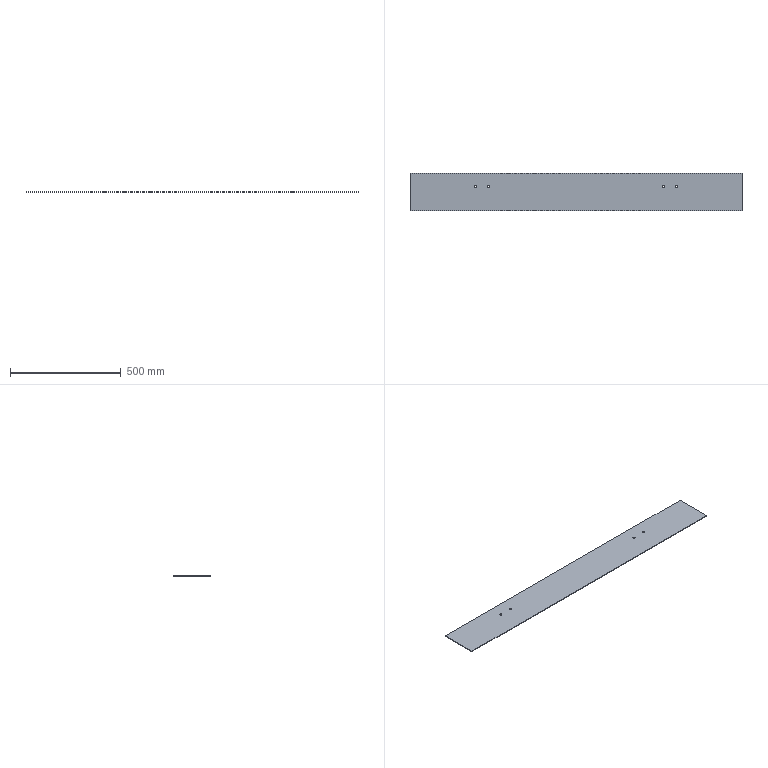Part | SolidWorks | features ICE 2, Extrusion 1, MirrorPattern 1 | 1 solid | 14 faces | box 1500 x 170 x 3 mm | volume 764058 mm3 | cylinder 8 | plane 6 | commonest cylinder face diameters 10 x8
STEP:
#1=CARTESIAN_POINT('',(400.26,30.,0.));
#2=VERTEX_POINT('',#1);
#3=CARTESIAN_POINT('',(390.26,30.,0.));
#4=VERTEX_POINT('',#3);
#5=CARTESIAN_POINT('',(395.26,30.,0.));
#6=DIRECTION('',(0.,0.,-1.));
#7=DIRECTION('',(-1.,0.,0.));
#8=AXIS2_PLACEMENT_3D('',#5,#6,#7);
#9=CIRCLE('',#8,5.);
#10=EDGE_CURVE('',#2,#4,#9,.T.);
#11=ORIENTED_EDGE('',*,*,#10,.T.);
#12=CARTESIAN_POINT('',(390.26,30.,3.));
#13=VERTEX_POINT('',#12);
#14=CARTESIAN_POINT('',(390.26,30.,0.));
#15=DIRECTION('',(0.,0.,1.));
#16=VECTOR('',#15,1000.);
#17=LINE('',#14,#16);
#18=EDGE_CURVE('',#4,#13,#17,.T.);
#19=ORIENTED_EDGE('',*,*,#18,.T.);
#20=CARTESIAN_POINT('',(400.26,30.,3.));
#21=VERTEX_POINT('',#20);
#22=CARTESIAN_POINT('',(395.26,30.,3.));
#23=DIRECTION('',(0.,0.,-1.));
#24=DIRECTION('',(-1.,0.,0.));
#25=AXIS2_PLACEMENT_3D('',#22,#23,#24);
#26=CIRCLE('',#25,5.);
#27=EDGE_CURVE('',#21,#13,#26,.T.);
#28=ORIENTED_EDGE('',*,*,#27,.F.);
#29=CARTESIAN_POINT('',(400.26,30.,0.));
#30=DIRECTION('',(0.,0.,1.));
#31=VECTOR('',#30,1000.);
#32=LINE('',#29,#31);
#33=EDGE_CURVE('',#2,#21,#32,.T.);
#34=ORIENTED_EDGE('',*,*,#33,.F.);
#35=EDGE_LOOP('',(#11,#19,#28,#34));
#36=FACE_OUTER_BOUND('',#35,.T.);
#37=CARTESIAN_POINT('',(395.26,30.,0.));
#38=DIRECTION('',(0.,0.,1.));
#39=DIRECTION('',(1.,0.,0.));
#40=AXIS2_PLACEMENT_3D('',#37,#38,#39);
#41=CYLINDRICAL_SURFACE('',#40,5.);
#42=ADVANCED_FACE('',(#36),#41,.F.);
#43=CARTESIAN_POINT('',(460.26,30.,0.));
#44=VERTEX_POINT('',#43);
#45=CARTESIAN_POINT('',(450.26,30.,0.));
#46=VERTEX_POINT('',#45);
#47=CARTESIAN_POINT('',(455.26,30.,0.));
#48=DIRECTION('',(0.,0.,-1.));
#49=DIRECTION('',(-1.,0.,0.));
#50=AXIS2_PLACEMENT_3D('',#47,#48,#49);
#51=CIRCLE('',#50,5.);
#52=EDGE_CURVE('',#44,#46,#51,.T.);
#53=ORIENTED_EDGE('',*,*,#52,.T.);
#54=CARTESIAN_POINT('',(450.26,30.,3.));
#55=VERTEX_POINT('',#54);
#56=CARTESIAN_POINT('',(450.26,30.,0.));
#57=DIRECTION('',(0.,0.,1.));
#58=VECTOR('',#57,1000.);
#59=LINE('',#56,#58);
#60=EDGE_CURVE('',#46,#55,#59,.T.);
#61=ORIENTED_EDGE('',*,*,#60,.T.);
#62=CARTESIAN_POINT('',(460.26,30.,3.));
#63=VERTEX_POINT('',#62);
#64=CARTESIAN_POINT('',(455.26,30.,3.));
#65=DIRECTION('',(0.,0.,-1.));
#66=DIRECTION('',(-1.,0.,0.));
#67=AXIS2_PLACEMENT_3D('',#64,#65,#66);
#68=CIRCLE('',#67,5.);
#69=EDGE_CURVE('',#63,#55,#68,.T.);
#70=ORIENTED_EDGE('',*,*,#69,.F.);
#71=CARTESIAN_POINT('',(460.26,30.,0.));
#72=DIRECTION('',(0.,0.,1.));
#73=VECTOR('',#72,1000.);
#74=LINE('',#71,#73);
#75=EDGE_CURVE('',#44,#63,#74,.T.);
#76=ORIENTED_EDGE('',*,*,#75,.F.);
#77=EDGE_LOOP('',(#53,#61,#70,#76));
#78=FACE_OUTER_BOUND('',#77,.T.);
#79=CARTESIAN_POINT('',(455.26,30.,0.));
#80=DIRECTION('',(0.,0.,1.));
#81=DIRECTION('',(1.,0.,0.));
#82=AXIS2_PLACEMENT_3D('',#79,#80,#81);
#83=CYLINDRICAL_SURFACE('',#82,5.);
#84=ADVANCED_FACE('',(#78),#83,.F.);
#85=CARTESIAN_POINT('',(-400.26,30.,0.));
#86=VERTEX_POINT('',#85);
#87=CARTESIAN_POINT('',(-390.26,30.,0.));
#88=VERTEX_POINT('',#87);
#89=CARTESIAN_POINT('',(-395.26,30.,0.));
#90=DIRECTION('',(0.,0.,1.));
#91=DIRECTION('',(1.,0.,0.));
#92=AXIS2_PLACEMENT_3D('',#89,#90,#91);
#93=CIRCLE('',#92,5.);
#94=EDGE_CURVE('',#86,#88,#93,.T.);
#95=ORIENTED_EDGE('',*,*,#94,.F.);
#96=CARTESIAN_POINT('',(-400.26,30.,3.));
#97=VERTEX_POINT('',#96);
#98=CARTESIAN_POINT('',(-400.26,30.,0.));
#99=DIRECTION('',(0.,0.,1.));
#100=VECTOR('',#99,1000.);
#101=LINE('',#98,#100);
#102=EDGE_CURVE('',#86,#97,#101,.T.);
#103=ORIENTED_EDGE('',*,*,#102,.T.);
#104=CARTESIAN_POINT('',(-390.26,30.,3.));
#105=VERTEX_POINT('',#104);
#106=CARTESIAN_POINT('',(-395.26,30.,3.));
#107=DIRECTION('',(0.,0.,1.));
#108=DIRECTION('',(1.,0.,0.));
#109=AXIS2_PLACEMENT_3D('',#106,#107,#108);
#110=CIRCLE('',#109,5.);
#111=EDGE_CURVE('',#97,#105,#110,.T.);
#112=ORIENTED_EDGE('',*,*,#111,.T.);
#113=CARTESIAN_POINT('',(-390.26,30.,0.));
#114=DIRECTION('',(0.,0.,1.));
#115=VECTOR('',#114,1000.);
#116=LINE('',#113,#115);
#117=EDGE_CURVE('',#88,#105,#116,.T.);
#118=ORIENTED_EDGE('',*,*,#117,.F.);
#119=EDGE_LOOP('',(#95,#103,#112,#118));
#120=FACE_OUTER_BOUND('',#119,.T.);
#121=CARTESIAN_POINT('',(-395.26,30.,0.));
#122=DIRECTION('',(0.,0.,1.));
#123=DIRECTION('',(1.,0.,0.));
#124=AXIS2_PLACEMENT_3D('',#121,#122,#123);
#125=CYLINDRICAL_SURFACE('',#124,5.);
#126=ADVANCED_FACE('',(#120),#125,.F.);
#127=CARTESIAN_POINT('',(-460.26,30.,0.));
#128=VERTEX_POINT('',#127);
#129=CARTESIAN_POINT('',(-450.26,30.,0.));
#130=VERTEX_POINT('',#129);
#131=CARTESIAN_POINT('',(-455.26,30.,0.));
#132=DIRECTION('',(0.,0.,1.));
#133=DIRECTION('',(1.,0.,0.));
#134=AXIS2_PLACEMENT_3D('',#131,#132,#133);
#135=CIRCLE('',#134,5.);
#136=EDGE_CURVE('',#128,#130,#135,.T.);
#137=ORIENTED_EDGE('',*,*,#136,.F.);
#138=CARTESIAN_POINT('',(-460.26,30.,3.));
#139=VERTEX_POINT('',#138);
#140=CARTESIAN_POINT('',(-460.26,30.,0.));
#141=DIRECTION('',(0.,0.,1.));
#142=VECTOR('',#141,1000.);
#143=LINE('',#140,#142);
#144=EDGE_CURVE('',#128,#139,#143,.T.);
#145=ORIENTED_EDGE('',*,*,#144,.T.);
#146=CARTESIAN_POINT('',(-450.26,30.,3.));
#147=VERTEX_POINT('',#146);
#148=CARTESIAN_POINT('',(-455.26,30.,3.));
#149=DIRECTION('',(0.,0.,1.));
#150=DIRECTION('',(1.,0.,0.));
#151=AXIS2_PLACEMENT_3D('',#148,#149,#150);
#152=CIRCLE('',#151,5.);
#153=EDGE_CURVE('',#139,#147,#152,.T.);
#154=ORIENTED_EDGE('',*,*,#153,.T.);
#155=CARTESIAN_POINT('',(-450.26,30.,0.));
#156=DIRECTION('',(0.,0.,1.));
#157=VECTOR('',#156,1000.);
#158=LINE('',#155,#157);
#159=EDGE_CURVE('',#130,#147,#158,.T.);
#160=ORIENTED_EDGE('',*,*,#159,.F.);
#161=EDGE_LOOP('',(#137,#145,#154,#160));
#162=FACE_OUTER_BOUND('',#161,.T.);
#163=CARTESIAN_POINT('',(-455.26,30.,0.));
#164=DIRECTION('',(0.,0.,1.));
#165=DIRECTION('',(1.,0.,0.));
#166=AXIS2_PLACEMENT_3D('',#163,#164,#165);
#167=CYLINDRICAL_SURFACE('',#166,5.);
#168=ADVANCED_FACE('',(#162),#167,.F.);
#169=CARTESIAN_POINT('',(750.,-80.,0.));
#170=VERTEX_POINT('',#169);
#171=CARTESIAN_POINT('',(750.,90.,0.));
#172=VERTEX_POINT('',#171);
#173=CARTESIAN_POINT('',(750.,-80.,0.));
#174=DIRECTION('',(0.,1.,0.));
#175=VECTOR('',#174,1000.);
#176=LINE('',#173,#175);
#177=EDGE_CURVE('',#170,#172,#176,.T.);
#178=ORIENTED_EDGE('',*,*,#177,.T.);
#179=CARTESIAN_POINT('',(750.,90.,3.));
#180=VERTEX_POINT('',#179);
#181=CARTESIAN_POINT('',(750.,90.,3.));
#182=DIRECTION('',(0.,0.,-1.));
#183=VECTOR('',#182,1000.);
#184=LINE('',#181,#183);
#185=EDGE_CURVE('',#180,#172,#184,.T.);
#186=ORIENTED_EDGE('',*,*,#185,.F.);
#187=CARTESIAN_POINT('',(750.,-80.,3.));
#188=VERTEX_POINT('',#187);
#189=CARTESIAN_POINT('',(750.,-80.,3.));
#190=DIRECTION('',(0.,1.,0.));
#191=VECTOR('',#190,1000.);
#192=LINE('',#189,#191);
#193=EDGE_CURVE('',#188,#180,#192,.T.);
#194=ORIENTED_EDGE('',*,*,#193,.F.);
#195=CARTESIAN_POINT('',(750.,-80.,3.));
#196=DIRECTION('',(0.,0.,-1.));
#197=VECTOR('',#196,1000.);
#198=LINE('',#195,#197);
#199=EDGE_CURVE('',#188,#170,#198,.T.);
#200=ORIENTED_EDGE('',*,*,#199,.T.);
#201=EDGE_LOOP('',(#178,#186,#194,#200));
#202=FACE_OUTER_BOUND('',#201,.T.);
#203=CARTESIAN_POINT('',(750.,-80.,3.));
#204=DIRECTION('',(-1.,0.,0.));
#205=DIRECTION('',(0.,0.,1.));
#206=AXIS2_PLACEMENT_3D('',#203,#204,#205);
#207=PLANE('',#206);
#208=ADVANCED_FACE('',(#202),#207,.F.);
#209=CARTESIAN_POINT('',(-750.,90.,0.));
#210=VERTEX_POINT('',#209);
#211=CARTESIAN_POINT('',(-750.,-80.,0.));
#212=VERTEX_POINT('',#211);
#213=CARTESIAN_POINT('',(-750.,-80.,0.));
#214=DIRECTION('',(0.,-1.,0.));
#215=VECTOR('',#214,1000.);
#216=LINE('',#213,#215);
#217=EDGE_CURVE('',#210,#212,#216,.T.);
#218=ORIENTED_EDGE('',*,*,#217,.T.);
#219=CARTESIAN_POINT('',(-750.,-80.,3.));
#220=VERTEX_POINT('',#219);
#221=CARTESIAN_POINT('',(-750.,-80.,3.));
#222=DIRECTION('',(0.,0.,-1.));
#223=VECTOR('',#222,1000.);
#224=LINE('',#221,#223);
#225=EDGE_CURVE('',#220,#212,#224,.T.);
#226=ORIENTED_EDGE('',*,*,#225,.F.);
#227=CARTESIAN_POINT('',(-750.,90.,3.));
#228=VERTEX_POINT('',#227);
#229=CARTESIAN_POINT('',(-750.,-80.,3.));
#230=DIRECTION('',(0.,-1.,0.));
#231=VECTOR('',#230,1000.);
#232=LINE('',#229,#231);
#233=EDGE_CURVE('',#228,#220,#232,.T.);
#234=ORIENTED_EDGE('',*,*,#233,.F.);
#235=CARTESIAN_POINT('',(-750.,90.,0.));
#236=DIRECTION('',(0.,0.,1.));
#237=VECTOR('',#236,1000.);
#238=LINE('',#235,#237);
#239=EDGE_CURVE('',#210,#228,#238,.T.);
#240=ORIENTED_EDGE('',*,*,#239,.F.);
#241=EDGE_LOOP('',(#218,#226,#234,#240));
#242=FACE_OUTER_BOUND('',#241,.T.);
#243=CARTESIAN_POINT('',(-750.,-80.,3.));
#244=DIRECTION('',(1.,0.,0.));
#245=DIRECTION('',(0.,0.,-1.));
#246=AXIS2_PLACEMENT_3D('',#243,#244,#245);
#247=PLANE('',#246);
#248=ADVANCED_FACE('',(#242),#247,.F.);
#249=CARTESIAN_POINT('',(-750.,-80.,0.));
#250=DIRECTION('',(1.,0.,0.));
#251=VECTOR('',#250,1000.);
#252=LINE('',#249,#251);
#253=EDGE_CURVE('',#212,#170,#252,.T.);
#254=ORIENTED_EDGE('',*,*,#253,.T.);
#255=ORIENTED_EDGE('',*,*,#199,.F.);
#256=CARTESIAN_POINT('',(-750.,-80.,3.));
#257=DIRECTION('',(1.,0.,0.));
#258=VECTOR('',#257,1000.);
#259=LINE('',#256,#258);
#260=EDGE_CURVE('',#220,#188,#259,.T.);
#261=ORIENTED_EDGE('',*,*,#260,.F.);
#262=ORIENTED_EDGE('',*,*,#225,.T.);
#263=EDGE_LOOP('',(#254,#255,#261,#262));
#264=FACE_OUTER_BOUND('',#263,.T.);
#265=CARTESIAN_POINT('',(-750.,-80.,3.));
#266=DIRECTION('',(0.,1.,0.));
#267=DIRECTION('',(0.,0.,1.));
#268=AXIS2_PLACEMENT_3D('',#265,#266,#267);
#269=PLANE('',#268);
#270=ADVANCED_FACE('',(#264),#269,.F.);
#271=ORIENTED_EDGE('',*,*,#27,.T.);
#272=CARTESIAN_POINT('',(395.26,30.,3.));
#273=DIRECTION('',(0.,0.,-1.));
#274=DIRECTION('',(-1.,0.,0.));
#275=AXIS2_PLACEMENT_3D('',#272,#273,#274);
#276=CIRCLE('',#275,5.);
#277=EDGE_CURVE('',#13,#21,#276,.T.);
#278=ORIENTED_EDGE('',*,*,#277,.T.);
#279=EDGE_LOOP('',(#271,#278));
#280=FACE_BOUND('',#279,.T.);
#281=ORIENTED_EDGE('',*,*,#69,.T.);
#282=CARTESIAN_POINT('',(455.26,30.,3.));
#283=DIRECTION('',(0.,0.,-1.));
#284=DIRECTION('',(-1.,0.,0.));
#285=AXIS2_PLACEMENT_3D('',#282,#283,#284);
#286=CIRCLE('',#285,5.);
#287=EDGE_CURVE('',#55,#63,#286,.T.);
#288=ORIENTED_EDGE('',*,*,#287,.T.);
#289=EDGE_LOOP('',(#281,#288));
#290=FACE_BOUND('',#289,.T.);
#291=CARTESIAN_POINT('',(-395.26,30.,3.));
#292=DIRECTION('',(0.,0.,1.));
#293=DIRECTION('',(1.,0.,0.));
#294=AXIS2_PLACEMENT_3D('',#291,#292,#293);
#295=CIRCLE('',#294,5.);
#296=EDGE_CURVE('',#105,#97,#295,.T.);
#297=ORIENTED_EDGE('',*,*,#296,.F.);
#298=ORIENTED_EDGE('',*,*,#111,.F.);
#299=EDGE_LOOP('',(#297,#298));
#300=FACE_BOUND('',#299,.T.);
#301=CARTESIAN_POINT('',(-455.26,30.,3.));
#302=DIRECTION('',(0.,0.,1.));
#303=DIRECTION('',(1.,0.,0.));
#304=AXIS2_PLACEMENT_3D('',#301,#302,#303);
#305=CIRCLE('',#304,5.);
#306=EDGE_CURVE('',#147,#139,#305,.T.);
#307=ORIENTED_EDGE('',*,*,#306,.F.);
#308=ORIENTED_EDGE('',*,*,#153,.F.);
#309=EDGE_LOOP('',(#307,#308));
#310=FACE_BOUND('',#309,.T.);
#311=ORIENTED_EDGE('',*,*,#193,.T.);
#312=CARTESIAN_POINT('',(-750.,90.,3.));
#313=DIRECTION('',(1.,0.,0.));
#314=VECTOR('',#313,1000.);
#315=LINE('',#312,#314);
#316=EDGE_CURVE('',#228,#180,#315,.T.);
#317=ORIENTED_EDGE('',*,*,#316,.F.);
#318=ORIENTED_EDGE('',*,*,#233,.T.);
#319=ORIENTED_EDGE('',*,*,#260,.T.);
#320=EDGE_LOOP('',(#311,#317,#318,#319));
#321=FACE_OUTER_BOUND('',#320,.T.);
#322=CARTESIAN_POINT('',(0.,0.,3.));
#323=DIRECTION('',(0.,0.,-1.));
#324=DIRECTION('',(-1.,0.,0.));
#325=AXIS2_PLACEMENT_3D('',#322,#323,#324);
#326=PLANE('',#325);
#327=ADVANCED_FACE('',(#280,#290,#300,#310,#321),#326,.F.);
#328=ORIENTED_EDGE('',*,*,#10,.F.);
#329=CARTESIAN_POINT('',(395.26,30.,0.));
#330=DIRECTION('',(0.,0.,-1.));
#331=DIRECTION('',(-1.,0.,0.));
#332=AXIS2_PLACEMENT_3D('',#329,#330,#331);
#333=CIRCLE('',#332,5.);
#334=EDGE_CURVE('',#4,#2,#333,.T.);
#335=ORIENTED_EDGE('',*,*,#334,.F.);
#336=EDGE_LOOP('',(#328,#335));
#337=FACE_BOUND('',#336,.T.);
#338=ORIENTED_EDGE('',*,*,#52,.F.);
#339=CARTESIAN_POINT('',(455.26,30.,0.));
#340=DIRECTION('',(0.,0.,-1.));
#341=DIRECTION('',(-1.,0.,0.));
#342=AXIS2_PLACEMENT_3D('',#339,#340,#341);
#343=CIRCLE('',#342,5.);
#344=EDGE_CURVE('',#46,#44,#343,.T.);
#345=ORIENTED_EDGE('',*,*,#344,.F.);
#346=EDGE_LOOP('',(#338,#345));
#347=FACE_BOUND('',#346,.T.);
#348=CARTESIAN_POINT('',(-395.26,30.,0.));
#349=DIRECTION('',(0.,0.,1.));
#350=DIRECTION('',(1.,0.,0.));
#351=AXIS2_PLACEMENT_3D('',#348,#349,#350);
#352=CIRCLE('',#351,5.);
#353=EDGE_CURVE('',#88,#86,#352,.T.);
#354=ORIENTED_EDGE('',*,*,#353,.T.);
#355=ORIENTED_EDGE('',*,*,#94,.T.);
#356=EDGE_LOOP('',(#354,#355));
#357=FACE_BOUND('',#356,.T.);
#358=CARTESIAN_POINT('',(-455.26,30.,0.));
#359=DIRECTION('',(0.,0.,1.));
#360=DIRECTION('',(1.,0.,0.));
#361=AXIS2_PLACEMENT_3D('',#358,#359,#360);
#362=CIRCLE('',#361,5.);
#363=EDGE_CURVE('',#130,#128,#362,.T.);
#364=ORIENTED_EDGE('',*,*,#363,.T.);
#365=ORIENTED_EDGE('',*,*,#136,.T.);
#366=EDGE_LOOP('',(#364,#365));
#367=FACE_BOUND('',#366,.T.);
#368=ORIENTED_EDGE('',*,*,#177,.F.);
#369=ORIENTED_EDGE('',*,*,#253,.F.);
#370=ORIENTED_EDGE('',*,*,#217,.F.);
#371=CARTESIAN_POINT('',(750.,90.,0.));
#372=DIRECTION('',(-1.,0.,0.));
#373=VECTOR('',#372,1000.);
#374=LINE('',#371,#373);
#375=EDGE_CURVE('',#172,#210,#374,.T.);
#376=ORIENTED_EDGE('',*,*,#375,.F.);
#377=EDGE_LOOP('',(#368,#369,#370,#376));
#378=FACE_OUTER_BOUND('',#377,.T.);
#379=CARTESIAN_POINT('',(0.,0.,0.));
#380=DIRECTION('',(0.,0.,-1.));
#381=DIRECTION('',(-1.,0.,0.));
#382=AXIS2_PLACEMENT_3D('',#379,#380,#381);
#383=PLANE('',#382);
#384=ADVANCED_FACE('',(#337,#347,#357,#367,#378),#383,.T.);
#385=ORIENTED_EDGE('',*,*,#144,.F.);
#386=ORIENTED_EDGE('',*,*,#363,.F.);
#387=ORIENTED_EDGE('',*,*,#159,.T.);
#388=ORIENTED_EDGE('',*,*,#306,.T.);
#389=EDGE_LOOP('',(#385,#386,#387,#388));
#390=FACE_OUTER_BOUND('',#389,.T.);
#391=CARTESIAN_POINT('',(-455.26,30.,0.));
#392=DIRECTION('',(0.,0.,1.));
#393=DIRECTION('',(1.,0.,0.));
#394=AXIS2_PLACEMENT_3D('',#391,#392,#393);
#395=CYLINDRICAL_SURFACE('',#394,5.);
#396=ADVANCED_FACE('',(#390),#395,.F.);
#397=ORIENTED_EDGE('',*,*,#102,.F.);
#398=ORIENTED_EDGE('',*,*,#353,.F.);
#399=ORIENTED_EDGE('',*,*,#117,.T.);
#400=ORIENTED_EDGE('',*,*,#296,.T.);
#401=EDGE_LOOP('',(#397,#398,#399,#400));
#402=FACE_OUTER_BOUND('',#401,.T.);
#403=CARTESIAN_POINT('',(-395.26,30.,0.));
#404=DIRECTION('',(0.,0.,1.));
#405=DIRECTION('',(1.,0.,0.));
#406=AXIS2_PLACEMENT_3D('',#403,#404,#405);
#407=CYLINDRICAL_SURFACE('',#406,5.);
#408=ADVANCED_FACE('',(#402),#407,.F.);
#409=ORIENTED_EDGE('',*,*,#60,.F.);
#410=ORIENTED_EDGE('',*,*,#344,.T.);
#411=ORIENTED_EDGE('',*,*,#75,.T.);
#412=ORIENTED_EDGE('',*,*,#287,.F.);
#413=EDGE_LOOP('',(#409,#410,#411,#412));
#414=FACE_OUTER_BOUND('',#413,.T.);
#415=CARTESIAN_POINT('',(455.26,30.,0.));
#416=DIRECTION('',(0.,0.,1.));
#417=DIRECTION('',(1.,0.,0.));
#418=AXIS2_PLACEMENT_3D('',#415,#416,#417);
#419=CYLINDRICAL_SURFACE('',#418,5.);
#420=ADVANCED_FACE('',(#414),#419,.F.);
#421=ORIENTED_EDGE('',*,*,#18,.F.);
#422=ORIENTED_EDGE('',*,*,#334,.T.);
#423=ORIENTED_EDGE('',*,*,#33,.T.);
#424=ORIENTED_EDGE('',*,*,#277,.F.);
#425=EDGE_LOOP('',(#421,#422,#423,#424));
#426=FACE_OUTER_BOUND('',#425,.T.);
#427=CARTESIAN_POINT('',(395.26,30.,0.));
#428=DIRECTION('',(0.,0.,1.));
#429=DIRECTION('',(1.,0.,0.));
#430=AXIS2_PLACEMENT_3D('',#427,#428,#429);
#431=CYLINDRICAL_SURFACE('',#430,5.);
#432=ADVANCED_FACE('',(#426),#431,.F.);
#433=ORIENTED_EDGE('',*,*,#185,.T.);
#434=ORIENTED_EDGE('',*,*,#375,.T.);
#435=ORIENTED_EDGE('',*,*,#239,.T.);
#436=ORIENTED_EDGE('',*,*,#316,.T.);
#437=EDGE_LOOP('',(#433,#434,#435,#436));
#438=FACE_OUTER_BOUND('',#437,.T.);
#439=CARTESIAN_POINT('',(0.,90.,0.));
#440=DIRECTION('',(0.,1.,0.));
#441=DIRECTION('',(0.,0.,1.));
#442=AXIS2_PLACEMENT_3D('',#439,#440,#441);
#443=PLANE('',#442);
#444=ADVANCED_FACE('',(#438),#443,.T.);
#445=CLOSED_SHELL('',(#42,#84,#126,#168,#208,#248,#270,#327,#384,#396,#408,#420,#432,#444));
#446=MANIFOLD_SOLID_BREP('',#445);
#447=CARTESIAN_POINT('',(0.,0.,0.));
#448=DIRECTION('',(0.,0.,1.));
#449=DIRECTION('',(1.,0.,0.));
#450=AXIS2_PLACEMENT_3D('',#447,#448,#449);
#451=(LENGTH_UNIT()NAMED_UNIT(*)SI_UNIT(.MILLI.,.METRE.));
#452=UNCERTAINTY_MEASURE_WITH_UNIT(LENGTH_MEASURE(0.00001),#451,'','');
#453=(NAMED_UNIT(*)PLANE_ANGLE_UNIT()SI_UNIT($,.RADIAN.));
#454=(NAMED_UNIT(*)SI_UNIT($,.STERADIAN.)SOLID_ANGLE_UNIT());
#455=(GEOMETRIC_REPRESENTATION_CONTEXT(3)GLOBAL_UNCERTAINTY_ASSIGNED_CONTEXT((#452))GLOBAL_UNIT_ASSIGNED_CONTEXT((#451,#453,#454))REPRESENTATION_CONTEXT('',''));
#456=ADVANCED_BREP_SHAPE_REPRESENTATION('',(#446,#450),#455);